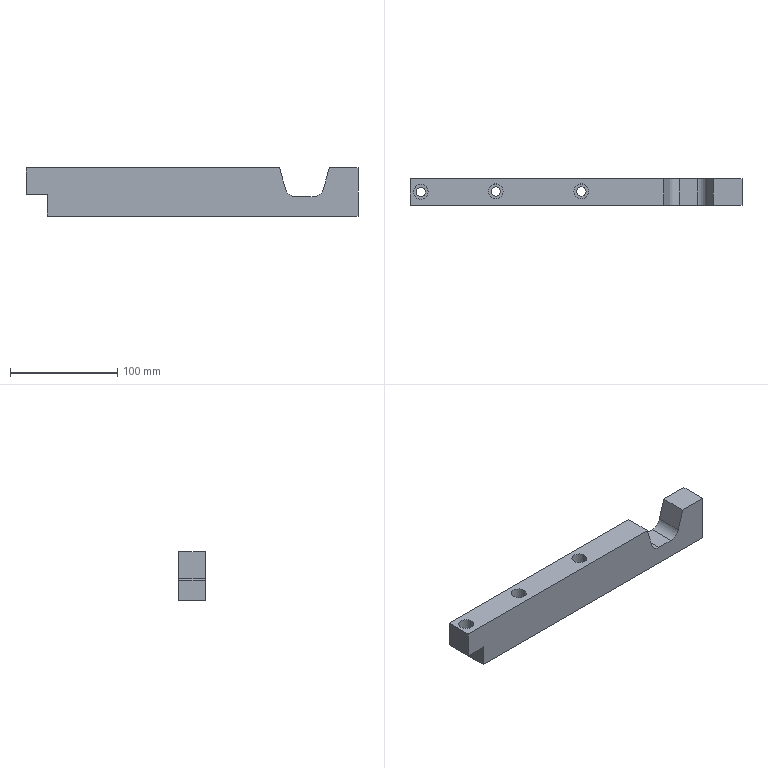Part | STEP file | 冲床-300配套压波_id986_x_t | 1 solid | 26 faces | box 310 x 25 x 45 mm | volume 301509 mm3 | plane 15 | cylinder 11 | commonest cylinder face diameters 8.7 x3 14 x3 4 x2 20 x2 1 x1
STEP:
#1=CARTESIAN_POINT('',(1952.,-82.5,-185.));
#2=VERTEX_POINT('',#1);
#3=CARTESIAN_POINT('',(1945.,-82.5,-185.));
#4=DIRECTION('',(0.,0.,-1.));
#5=DIRECTION('',(1.,0.,0.));
#6=AXIS2_PLACEMENT_3D('',#3,#4,#5);
#7=CIRCLE('',#6,7.);
#8=EDGE_CURVE('',#2,#2,#7,.T.);
#9=ORIENTED_EDGE('',*,*,#8,.T.);
#10=EDGE_LOOP('',(#9));
#11=FACE_BOUND('',#10,.T.);
#12=CARTESIAN_POINT('',(2102.,-82.01,-185.));
#13=VERTEX_POINT('',#12);
#14=CARTESIAN_POINT('',(2095.,-82.01,-185.));
#15=DIRECTION('',(0.,0.,-1.));
#16=DIRECTION('',(1.,0.,0.));
#17=AXIS2_PLACEMENT_3D('',#14,#15,#16);
#18=CIRCLE('',#17,7.);
#19=EDGE_CURVE('',#13,#13,#18,.T.);
#20=ORIENTED_EDGE('',*,*,#19,.T.);
#21=EDGE_LOOP('',(#20));
#22=FACE_BOUND('',#21,.T.);
#23=CARTESIAN_POINT('',(2022.,-82.01,-185.));
#24=VERTEX_POINT('',#23);
#25=CARTESIAN_POINT('',(2015.,-82.01,-185.));
#26=DIRECTION('',(0.,0.,-1.));
#27=DIRECTION('',(1.,0.,0.));
#28=AXIS2_PLACEMENT_3D('',#25,#26,#27);
#29=CIRCLE('',#28,7.);
#30=EDGE_CURVE('',#24,#24,#29,.T.);
#31=ORIENTED_EDGE('',*,*,#30,.T.);
#32=EDGE_LOOP('',(#31));
#33=FACE_BOUND('',#32,.T.);
#34=CARTESIAN_POINT('',(2171.709,-95.,-185.));
#35=VERTEX_POINT('',#34);
#36=CARTESIAN_POINT('',(1935.,-95.,-185.));
#37=VERTEX_POINT('',#36);
#38=CARTESIAN_POINT('',(1985.,-95.,-185.));
#39=DIRECTION('',(-1.,0.,0.));
#40=VECTOR('',#39,1.);
#41=LINE('',#38,#40);
#42=EDGE_CURVE('',#35,#37,#41,.T.);
#43=ORIENTED_EDGE('',*,*,#42,.F.);
#44=CARTESIAN_POINT('',(2171.709,-70.,-185.));
#45=VERTEX_POINT('',#44);
#46=CARTESIAN_POINT('',(2171.709,-298.,-185.));
#47=DIRECTION('',(0.,1.,0.));
#48=VECTOR('',#47,1.);
#49=LINE('',#46,#48);
#50=EDGE_CURVE('',#35,#45,#49,.T.);
#51=ORIENTED_EDGE('',*,*,#50,.T.);
#52=CARTESIAN_POINT('',(1935.,-70.,-185.));
#53=VERTEX_POINT('',#52);
#54=CARTESIAN_POINT('',(2135.,-70.,-185.));
#55=DIRECTION('',(-1.,0.,0.));
#56=VECTOR('',#55,1.);
#57=LINE('',#54,#56);
#58=EDGE_CURVE('',#45,#53,#57,.T.);
#59=ORIENTED_EDGE('',*,*,#58,.T.);
#60=CARTESIAN_POINT('',(1935.,-298.,-185.));
#61=DIRECTION('',(0.,-1.,0.));
#62=VECTOR('',#61,1.);
#63=LINE('',#60,#62);
#64=EDGE_CURVE('',#53,#37,#63,.T.);
#65=ORIENTED_EDGE('',*,*,#64,.T.);
#66=EDGE_LOOP('',(#43,#51,#59,#65));
#67=FACE_BOUND('',#66,.T.);
#68=CARTESIAN_POINT('',(1985.,-298.,-185.));
#69=DIRECTION('',(0.,0.,1.));
#70=DIRECTION('',(1.,0.,0.));
#71=AXIS2_PLACEMENT_3D('',#68,#69,#70);
#72=PLANE('',#71);
#73=ADVANCED_FACE('',(#11,#22,#33,#67),#72,.T.);
#74=CARTESIAN_POINT('',(2245.,-95.,-185.));
#75=VERTEX_POINT('',#74);
#76=CARTESIAN_POINT('',(2245.,-70.,-185.));
#77=VERTEX_POINT('',#76);
#78=CARTESIAN_POINT('',(2245.,-298.,-185.));
#79=DIRECTION('',(0.,1.,0.));
#80=VECTOR('',#79,1.);
#81=LINE('',#78,#80);
#82=EDGE_CURVE('',#75,#77,#81,.T.);
#83=ORIENTED_EDGE('',*,*,#82,.T.);
#84=CARTESIAN_POINT('',(2218.291,-70.,-185.));
#85=VERTEX_POINT('',#84);
#86=CARTESIAN_POINT('',(2135.,-70.,-185.));
#87=DIRECTION('',(-1.,0.,0.));
#88=VECTOR('',#87,1.);
#89=LINE('',#86,#88);
#90=EDGE_CURVE('',#77,#85,#89,.T.);
#91=ORIENTED_EDGE('',*,*,#90,.T.);
#92=CARTESIAN_POINT('',(2218.291,-95.,-185.));
#93=VERTEX_POINT('',#92);
#94=CARTESIAN_POINT('',(2218.291,-298.,-185.));
#95=DIRECTION('',(0.,-1.,0.));
#96=VECTOR('',#95,1.);
#97=LINE('',#94,#96);
#98=EDGE_CURVE('',#85,#93,#97,.T.);
#99=ORIENTED_EDGE('',*,*,#98,.T.);
#100=CARTESIAN_POINT('',(1975.,-95.,-185.));
#101=DIRECTION('',(-1.,0.,0.));
#102=VECTOR('',#101,1.);
#103=LINE('',#100,#102);
#104=EDGE_CURVE('',#75,#93,#103,.T.);
#105=ORIENTED_EDGE('',*,*,#104,.F.);
#106=EDGE_LOOP('',(#83,#91,#99,#105));
#107=FACE_OUTER_BOUND('',#106,.T.);
#108=CARTESIAN_POINT('',(1975.,-298.,-185.));
#109=DIRECTION('',(0.,0.,1.));
#110=DIRECTION('',(1.,0.,0.));
#111=AXIS2_PLACEMENT_3D('',#108,#109,#110);
#112=PLANE('',#111);
#113=ADVANCED_FACE('',(#107),#112,.T.);
#114=CARTESIAN_POINT('',(2245.,-95.,-230.));
#115=VERTEX_POINT('',#114);
#116=CARTESIAN_POINT('',(2245.,-70.,-230.));
#117=VERTEX_POINT('',#116);
#118=CARTESIAN_POINT('',(2245.,-298.,-230.));
#119=DIRECTION('',(0.,1.,0.));
#120=VECTOR('',#119,1.);
#121=LINE('',#118,#120);
#122=EDGE_CURVE('',#115,#117,#121,.T.);
#123=ORIENTED_EDGE('',*,*,#122,.T.);
#124=CARTESIAN_POINT('',(2245.,-70.,-390.));
#125=DIRECTION('',(0.,0.,1.));
#126=VECTOR('',#125,1.);
#127=LINE('',#124,#126);
#128=EDGE_CURVE('',#117,#77,#127,.T.);
#129=ORIENTED_EDGE('',*,*,#128,.T.);
#130=ORIENTED_EDGE('',*,*,#82,.F.);
#131=CARTESIAN_POINT('',(2245.,-95.,-190.));
#132=DIRECTION('',(0.,0.,1.));
#133=VECTOR('',#132,1.);
#134=LINE('',#131,#133);
#135=EDGE_CURVE('',#115,#75,#134,.T.);
#136=ORIENTED_EDGE('',*,*,#135,.F.);
#137=EDGE_LOOP('',(#123,#129,#130,#136));
#138=FACE_OUTER_BOUND('',#137,.T.);
#139=CARTESIAN_POINT('',(2245.,-298.,-190.));
#140=DIRECTION('',(1.,0.,0.));
#141=DIRECTION('',(0.,1.,0.));
#142=AXIS2_PLACEMENT_3D('',#139,#140,#141);
#143=PLANE('',#142);
#144=ADVANCED_FACE('',(#138),#143,.T.);
#145=CARTESIAN_POINT('',(1955.,-70.,-230.));
#146=VERTEX_POINT('',#145);
#147=CARTESIAN_POINT('',(1985.,-70.,-230.));
#148=DIRECTION('',(1.,0.,0.));
#149=VECTOR('',#148,1.);
#150=LINE('',#147,#149);
#151=EDGE_CURVE('',#146,#117,#150,.T.);
#152=ORIENTED_EDGE('',*,*,#151,.T.);
#153=ORIENTED_EDGE('',*,*,#122,.F.);
#154=CARTESIAN_POINT('',(1955.,-95.,-230.));
#155=VERTEX_POINT('',#154);
#156=CARTESIAN_POINT('',(1985.,-95.,-230.));
#157=DIRECTION('',(-1.,0.,0.));
#158=VECTOR('',#157,1.);
#159=LINE('',#156,#158);
#160=EDGE_CURVE('',#115,#155,#159,.T.);
#161=ORIENTED_EDGE('',*,*,#160,.T.);
#162=CARTESIAN_POINT('',(1955.,-80.,-230.));
#163=DIRECTION('',(0.,-1.,0.));
#164=VECTOR('',#163,1.);
#165=LINE('',#162,#164);
#166=EDGE_CURVE('',#146,#155,#165,.T.);
#167=ORIENTED_EDGE('',*,*,#166,.F.);
#168=EDGE_LOOP('',(#152,#153,#161,#167));
#169=FACE_BOUND('',#168,.T.);
#170=CARTESIAN_POINT('',(2019.35,-82.01,-230.));
#171=VERTEX_POINT('',#170);
#172=CARTESIAN_POINT('',(2015.,-82.01,-230.));
#173=DIRECTION('',(0.,0.,1.));
#174=DIRECTION('',(1.,0.,0.));
#175=AXIS2_PLACEMENT_3D('',#172,#173,#174);
#176=CIRCLE('',#175,4.35);
#177=EDGE_CURVE('',#171,#171,#176,.T.);
#178=ORIENTED_EDGE('',*,*,#177,.T.);
#179=EDGE_LOOP('',(#178));
#180=FACE_BOUND('',#179,.T.);
#181=CARTESIAN_POINT('',(2099.35,-82.01,-230.));
#182=VERTEX_POINT('',#181);
#183=CARTESIAN_POINT('',(2095.,-82.01,-230.));
#184=DIRECTION('',(0.,0.,1.));
#185=DIRECTION('',(1.,0.,0.));
#186=AXIS2_PLACEMENT_3D('',#183,#184,#185);
#187=CIRCLE('',#186,4.35);
#188=EDGE_CURVE('',#182,#182,#187,.T.);
#189=ORIENTED_EDGE('',*,*,#188,.T.);
#190=EDGE_LOOP('',(#189));
#191=FACE_BOUND('',#190,.T.);
#192=CARTESIAN_POINT('',(1985.,-298.,-230.));
#193=DIRECTION('',(0.,0.,1.));
#194=DIRECTION('',(1.,0.,0.));
#195=AXIS2_PLACEMENT_3D('',#192,#193,#194);
#196=PLANE('',#195);
#197=ADVANCED_FACE('',(#169,#180,#191),#196,.F.);
#198=CARTESIAN_POINT('',(1955.,-95.,-211.5));
#199=VERTEX_POINT('',#198);
#200=CARTESIAN_POINT('',(1955.,-95.,-70.));
#201=DIRECTION('',(0.,0.,1.));
#202=VECTOR('',#201,1.);
#203=LINE('',#200,#202);
#204=EDGE_CURVE('',#155,#199,#203,.T.);
#205=ORIENTED_EDGE('',*,*,#204,.T.);
#206=CARTESIAN_POINT('',(1955.,-70.,-211.5));
#207=VERTEX_POINT('',#206);
#208=CARTESIAN_POINT('',(1955.,0.,-211.5));
#209=DIRECTION('',(0.,1.,0.));
#210=VECTOR('',#209,1.);
#211=LINE('',#208,#210);
#212=EDGE_CURVE('',#199,#207,#211,.T.);
#213=ORIENTED_EDGE('',*,*,#212,.T.);
#214=CARTESIAN_POINT('',(1955.,-70.,-390.));
#215=DIRECTION('',(0.,0.,-1.));
#216=VECTOR('',#215,1.);
#217=LINE('',#214,#216);
#218=EDGE_CURVE('',#207,#146,#217,.T.);
#219=ORIENTED_EDGE('',*,*,#218,.T.);
#220=ORIENTED_EDGE('',*,*,#166,.T.);
#221=EDGE_LOOP('',(#205,#213,#219,#220));
#222=FACE_OUTER_BOUND('',#221,.T.);
#223=CARTESIAN_POINT('',(1955.,0.,-312.5));
#224=DIRECTION('',(-1.,0.,0.));
#225=DIRECTION('',(0.,0.,1.));
#226=AXIS2_PLACEMENT_3D('',#223,#224,#225);
#227=PLANE('',#226);
#228=ADVANCED_FACE('',(#222),#227,.T.);
#229=CARTESIAN_POINT('',(2212.604,-70.,-204.765));
#230=VERTEX_POINT('',#229);
#231=CARTESIAN_POINT('',(2225.867,-70.,-158.668));
#232=DIRECTION('',(-0.2765,0.,-0.961));
#233=VECTOR('',#232,1.);
#234=LINE('',#231,#233);
#235=EDGE_CURVE('',#85,#230,#234,.T.);
#236=ORIENTED_EDGE('',*,*,#235,.F.);
#237=ORIENTED_EDGE('',*,*,#90,.F.);
#238=ORIENTED_EDGE('',*,*,#128,.F.);
#239=ORIENTED_EDGE('',*,*,#151,.F.);
#240=ORIENTED_EDGE('',*,*,#218,.F.);
#241=CARTESIAN_POINT('',(1955.4,-70.,-210.3));
#242=VERTEX_POINT('',#241);
#243=CARTESIAN_POINT('',(1957.,-70.,-211.5));
#244=DIRECTION('',(0.,1.,0.));
#245=DIRECTION('',(0.,0.,-1.));
#246=AXIS2_PLACEMENT_3D('',#243,#244,#245);
#247=CIRCLE('',#246,2.);
#248=EDGE_CURVE('',#207,#242,#247,.T.);
#249=ORIENTED_EDGE('',*,*,#248,.T.);
#250=CARTESIAN_POINT('',(1954.7,-70.,-209.6));
#251=VERTEX_POINT('',#250);
#252=CARTESIAN_POINT('',(1955.,-70.,-210.));
#253=DIRECTION('',(0.,1.,0.));
#254=DIRECTION('',(-1.,0.,0.));
#255=AXIS2_PLACEMENT_3D('',#252,#253,#254);
#256=CIRCLE('',#255,0.5);
#257=EDGE_CURVE('',#251,#242,#256,.T.);
#258=ORIENTED_EDGE('',*,*,#257,.F.);
#259=CARTESIAN_POINT('',(1953.5,-70.,-210.));
#260=VERTEX_POINT('',#259);
#261=CARTESIAN_POINT('',(1953.5,-70.,-208.));
#262=DIRECTION('',(0.,1.,0.));
#263=DIRECTION('',(0.,0.,-1.));
#264=AXIS2_PLACEMENT_3D('',#261,#262,#263);
#265=CIRCLE('',#264,2.);
#266=EDGE_CURVE('',#251,#260,#265,.T.);
#267=ORIENTED_EDGE('',*,*,#266,.T.);
#268=CARTESIAN_POINT('',(1935.,-70.,-210.));
#269=VERTEX_POINT('',#268);
#270=CARTESIAN_POINT('',(1955.,-70.,-210.));
#271=DIRECTION('',(-1.,0.,0.));
#272=VECTOR('',#271,1.);
#273=LINE('',#270,#272);
#274=EDGE_CURVE('',#260,#269,#273,.T.);
#275=ORIENTED_EDGE('',*,*,#274,.T.);
#276=CARTESIAN_POINT('',(1935.,-70.,-185.));
#277=DIRECTION('',(0.,0.,-1.));
#278=VECTOR('',#277,1.);
#279=LINE('',#276,#278);
#280=EDGE_CURVE('',#53,#269,#279,.T.);
#281=ORIENTED_EDGE('',*,*,#280,.F.);
#282=ORIENTED_EDGE('',*,*,#58,.F.);
#283=CARTESIAN_POINT('',(2177.396,-70.,-204.765));
#284=VERTEX_POINT('',#283);
#285=CARTESIAN_POINT('',(2180.341,-70.,-215.));
#286=DIRECTION('',(-0.2765,0.,0.961));
#287=VECTOR('',#286,1.);
#288=LINE('',#285,#287);
#289=EDGE_CURVE('',#284,#45,#288,.T.);
#290=ORIENTED_EDGE('',*,*,#289,.F.);
#291=CARTESIAN_POINT('',(2187.006,-70.,-212.));
#292=VERTEX_POINT('',#291);
#293=CARTESIAN_POINT('',(2187.006,-70.,-202.));
#294=DIRECTION('',(0.,-1.,0.));
#295=DIRECTION('',(0.,0.,-1.));
#296=AXIS2_PLACEMENT_3D('',#293,#294,#295);
#297=CIRCLE('',#296,10.);
#298=EDGE_CURVE('',#284,#292,#297,.T.);
#299=ORIENTED_EDGE('',*,*,#298,.T.);
#300=CARTESIAN_POINT('',(2202.994,-70.,-212.));
#301=VERTEX_POINT('',#300);
#302=CARTESIAN_POINT('',(2135.,-70.,-212.));
#303=DIRECTION('',(-1.,0.,0.));
#304=VECTOR('',#303,1.);
#305=LINE('',#302,#304);
#306=EDGE_CURVE('',#301,#292,#305,.T.);
#307=ORIENTED_EDGE('',*,*,#306,.F.);
#308=CARTESIAN_POINT('',(2202.994,-70.,-202.));
#309=DIRECTION('',(0.,-1.,0.));
#310=DIRECTION('',(0.,0.,-1.));
#311=AXIS2_PLACEMENT_3D('',#308,#309,#310);
#312=CIRCLE('',#311,10.);
#313=EDGE_CURVE('',#301,#230,#312,.T.);
#314=ORIENTED_EDGE('',*,*,#313,.T.);
#315=EDGE_LOOP('',(#236,#237,#238,#239,#240,#249,#258,#267,#275,#281,#282,#290,#299,#307,#314));
#316=FACE_OUTER_BOUND('',#315,.T.);
#317=CARTESIAN_POINT('',(2135.,-70.,-390.));
#318=DIRECTION('',(0.,-1.,0.));
#319=DIRECTION('',(0.,0.,-1.));
#320=AXIS2_PLACEMENT_3D('',#317,#318,#319);
#321=PLANE('',#320);
#322=ADVANCED_FACE('',(#316),#321,.F.);
#323=ORIENTED_EDGE('',*,*,#104,.T.);
#324=CARTESIAN_POINT('',(2212.604,-95.,-204.765));
#325=VERTEX_POINT('',#324);
#326=CARTESIAN_POINT('',(2312.487,-95.,142.39));
#327=DIRECTION('',(-0.2765,0.,-0.961));
#328=VECTOR('',#327,1.);
#329=LINE('',#326,#328);
#330=EDGE_CURVE('',#93,#325,#329,.T.);
#331=ORIENTED_EDGE('',*,*,#330,.T.);
#332=CARTESIAN_POINT('',(2202.994,-95.,-212.));
#333=VERTEX_POINT('',#332);
#334=CARTESIAN_POINT('',(2202.994,-95.,-202.));
#335=DIRECTION('',(0.,1.,0.));
#336=DIRECTION('',(0.,0.,1.));
#337=AXIS2_PLACEMENT_3D('',#334,#335,#336);
#338=CIRCLE('',#337,10.);
#339=EDGE_CURVE('',#325,#333,#338,.T.);
#340=ORIENTED_EDGE('',*,*,#339,.T.);
#341=CARTESIAN_POINT('',(2187.006,-95.,-212.));
#342=VERTEX_POINT('',#341);
#343=CARTESIAN_POINT('',(2195.,-95.,-212.));
#344=DIRECTION('',(-1.,0.,0.));
#345=VECTOR('',#344,1.);
#346=LINE('',#343,#345);
#347=EDGE_CURVE('',#333,#342,#346,.T.);
#348=ORIENTED_EDGE('',*,*,#347,.T.);
#349=CARTESIAN_POINT('',(2177.396,-95.,-204.765));
#350=VERTEX_POINT('',#349);
#351=CARTESIAN_POINT('',(2187.006,-95.,-202.));
#352=DIRECTION('',(0.,1.,0.));
#353=DIRECTION('',(0.,0.,1.));
#354=AXIS2_PLACEMENT_3D('',#351,#352,#353);
#355=CIRCLE('',#354,10.);
#356=EDGE_CURVE('',#342,#350,#355,.T.);
#357=ORIENTED_EDGE('',*,*,#356,.T.);
#358=CARTESIAN_POINT('',(2164.133,-95.,-158.668));
#359=DIRECTION('',(-0.2765,0.,0.961));
#360=VECTOR('',#359,1.);
#361=LINE('',#358,#360);
#362=EDGE_CURVE('',#350,#35,#361,.T.);
#363=ORIENTED_EDGE('',*,*,#362,.T.);
#364=ORIENTED_EDGE('',*,*,#42,.T.);
#365=CARTESIAN_POINT('',(1935.,-95.,-210.));
#366=VERTEX_POINT('',#365);
#367=CARTESIAN_POINT('',(1935.,-95.,-185.));
#368=DIRECTION('',(0.,0.,-1.));
#369=VECTOR('',#368,1.);
#370=LINE('',#367,#369);
#371=EDGE_CURVE('',#37,#366,#370,.T.);
#372=ORIENTED_EDGE('',*,*,#371,.T.);
#373=CARTESIAN_POINT('',(1953.5,-95.,-210.));
#374=VERTEX_POINT('',#373);
#375=CARTESIAN_POINT('',(1975.,-95.,-210.));
#376=DIRECTION('',(-1.,0.,0.));
#377=VECTOR('',#376,1.);
#378=LINE('',#375,#377);
#379=EDGE_CURVE('',#374,#366,#378,.T.);
#380=ORIENTED_EDGE('',*,*,#379,.F.);
#381=CARTESIAN_POINT('',(1954.7,-95.,-209.6));
#382=VERTEX_POINT('',#381);
#383=CARTESIAN_POINT('',(1953.5,-95.,-208.));
#384=DIRECTION('',(0.,-1.,0.));
#385=DIRECTION('',(0.,0.,1.));
#386=AXIS2_PLACEMENT_3D('',#383,#384,#385);
#387=CIRCLE('',#386,2.);
#388=EDGE_CURVE('',#374,#382,#387,.T.);
#389=ORIENTED_EDGE('',*,*,#388,.T.);
#390=CARTESIAN_POINT('',(1955.4,-95.,-210.3));
#391=VERTEX_POINT('',#390);
#392=CARTESIAN_POINT('',(1955.,-95.,-210.));
#393=DIRECTION('',(0.,-1.,0.));
#394=DIRECTION('',(-1.,0.,0.));
#395=AXIS2_PLACEMENT_3D('',#392,#393,#394);
#396=CIRCLE('',#395,0.5);
#397=EDGE_CURVE('',#391,#382,#396,.T.);
#398=ORIENTED_EDGE('',*,*,#397,.F.);
#399=CARTESIAN_POINT('',(1957.,-95.,-211.5));
#400=DIRECTION('',(0.,-1.,0.));
#401=DIRECTION('',(0.,0.,1.));
#402=AXIS2_PLACEMENT_3D('',#399,#400,#401);
#403=CIRCLE('',#402,2.);
#404=EDGE_CURVE('',#391,#199,#403,.T.);
#405=ORIENTED_EDGE('',*,*,#404,.T.);
#406=ORIENTED_EDGE('',*,*,#204,.F.);
#407=ORIENTED_EDGE('',*,*,#160,.F.);
#408=ORIENTED_EDGE('',*,*,#135,.T.);
#409=EDGE_LOOP('',(#323,#331,#340,#348,#357,#363,#364,#372,#380,#389,#398,#405,#406,#407,#408));
#410=FACE_OUTER_BOUND('',#409,.T.);
#411=CARTESIAN_POINT('',(1975.,-95.,-70.));
#412=DIRECTION('',(0.,1.,0.));
#413=DIRECTION('',(0.,0.,1.));
#414=AXIS2_PLACEMENT_3D('',#411,#412,#413);
#415=PLANE('',#414);
#416=ADVANCED_FACE('',(#410),#415,.F.);
#417=CARTESIAN_POINT('',(1940.65,-82.5,-210.));
#418=VERTEX_POINT('',#417);
#419=CARTESIAN_POINT('',(1945.,-82.5,-210.));
#420=DIRECTION('',(0.,0.,-1.));
#421=DIRECTION('',(-1.,0.,0.));
#422=AXIS2_PLACEMENT_3D('',#419,#420,#421);
#423=CIRCLE('',#422,4.35);
#424=EDGE_CURVE('',#418,#418,#423,.T.);
#425=ORIENTED_EDGE('',*,*,#424,.F.);
#426=EDGE_LOOP('',(#425));
#427=FACE_BOUND('',#426,.T.);
#428=ORIENTED_EDGE('',*,*,#274,.F.);
#429=CARTESIAN_POINT('',(1953.5,-70.,-210.));
#430=DIRECTION('',(0.,-1.,0.));
#431=VECTOR('',#430,1.);
#432=LINE('',#429,#431);
#433=EDGE_CURVE('',#260,#374,#432,.T.);
#434=ORIENTED_EDGE('',*,*,#433,.T.);
#435=ORIENTED_EDGE('',*,*,#379,.T.);
#436=CARTESIAN_POINT('',(1935.,-70.,-210.));
#437=DIRECTION('',(0.,-1.,0.));
#438=VECTOR('',#437,1.);
#439=LINE('',#436,#438);
#440=EDGE_CURVE('',#269,#366,#439,.T.);
#441=ORIENTED_EDGE('',*,*,#440,.F.);
#442=EDGE_LOOP('',(#428,#434,#435,#441));
#443=FACE_BOUND('',#442,.T.);
#444=CARTESIAN_POINT('',(1955.,-70.,-210.));
#445=DIRECTION('',(0.,0.,-1.));
#446=DIRECTION('',(-1.,0.,0.));
#447=AXIS2_PLACEMENT_3D('',#444,#445,#446);
#448=PLANE('',#447);
#449=ADVANCED_FACE('',(#427,#443),#448,.T.);
#450=CARTESIAN_POINT('',(2090.65,-82.01,-205.));
#451=VERTEX_POINT('',#450);
#452=CARTESIAN_POINT('',(2095.,-82.01,-205.));
#453=DIRECTION('',(0.,0.,1.));
#454=DIRECTION('',(-1.,0.,0.));
#455=AXIS2_PLACEMENT_3D('',#452,#453,#454);
#456=CIRCLE('',#455,4.35);
#457=EDGE_CURVE('',#451,#451,#456,.T.);
#458=ORIENTED_EDGE('',*,*,#457,.F.);
#459=EDGE_LOOP('',(#458));
#460=FACE_BOUND('',#459,.T.);
#461=CARTESIAN_POINT('',(2088.,-82.01,-205.));
#462=VERTEX_POINT('',#461);
#463=CARTESIAN_POINT('',(2095.,-82.01,-205.));
#464=DIRECTION('',(0.,0.,1.));
#465=DIRECTION('',(-1.,0.,0.));
#466=AXIS2_PLACEMENT_3D('',#463,#464,#465);
#467=CIRCLE('',#466,7.);
#468=EDGE_CURVE('',#462,#462,#467,.T.);
#469=ORIENTED_EDGE('',*,*,#468,.T.);
#470=EDGE_LOOP('',(#469));
#471=FACE_BOUND('',#470,.T.);
#472=CARTESIAN_POINT('',(2095.,-82.01,-205.));
#473=DIRECTION('',(0.,0.,-1.));
#474=DIRECTION('',(-1.,0.,0.));
#475=AXIS2_PLACEMENT_3D('',#472,#473,#474);
#476=PLANE('',#475);
#477=ADVANCED_FACE('',(#460,#471),#476,.F.);
#478=ORIENTED_EDGE('',*,*,#19,.F.);
#479=EDGE_LOOP('',(#478));
#480=FACE_BOUND('',#479,.T.);
#481=ORIENTED_EDGE('',*,*,#468,.F.);
#482=EDGE_LOOP('',(#481));
#483=FACE_BOUND('',#482,.T.);
#484=CARTESIAN_POINT('',(2095.,-82.01,-185.));
#485=DIRECTION('',(0.,0.,-1.));
#486=DIRECTION('',(-1.,0.,0.));
#487=AXIS2_PLACEMENT_3D('',#484,#485,#486);
#488=CYLINDRICAL_SURFACE('',#487,7.);
#489=ADVANCED_FACE('',(#480,#483),#488,.F.);
#490=ORIENTED_EDGE('',*,*,#330,.F.);
#491=ORIENTED_EDGE('',*,*,#98,.F.);
#492=ORIENTED_EDGE('',*,*,#235,.T.);
#493=CARTESIAN_POINT('',(2212.604,-95.,-204.765));
#494=DIRECTION('',(0.,-1.,0.));
#495=VECTOR('',#494,1.);
#496=LINE('',#493,#495);
#497=EDGE_CURVE('',#230,#325,#496,.T.);
#498=ORIENTED_EDGE('',*,*,#497,.T.);
#499=EDGE_LOOP('',(#490,#491,#492,#498));
#500=FACE_OUTER_BOUND('',#499,.T.);
#501=CARTESIAN_POINT('',(2312.487,-70.,142.39));
#502=DIRECTION('',(-0.961,0.,0.2765));
#503=DIRECTION('',(0.2765,0.,0.961));
#504=AXIS2_PLACEMENT_3D('',#501,#502,#503);
#505=PLANE('',#504);
#506=ADVANCED_FACE('',(#500),#505,.T.);
#507=ORIENTED_EDGE('',*,*,#289,.T.);
#508=ORIENTED_EDGE('',*,*,#50,.F.);
#509=ORIENTED_EDGE('',*,*,#362,.F.);
#510=CARTESIAN_POINT('',(2177.396,-70.,-204.765));
#511=DIRECTION('',(0.,1.,0.));
#512=VECTOR('',#511,1.);
#513=LINE('',#510,#512);
#514=EDGE_CURVE('',#350,#284,#513,.T.);
#515=ORIENTED_EDGE('',*,*,#514,.T.);
#516=EDGE_LOOP('',(#507,#508,#509,#515));
#517=FACE_OUTER_BOUND('',#516,.T.);
#518=CARTESIAN_POINT('',(2164.133,-70.,-158.668));
#519=DIRECTION('',(0.961,0.,0.2765));
#520=DIRECTION('',(0.2765,0.,-0.961));
#521=AXIS2_PLACEMENT_3D('',#518,#519,#520);
#522=PLANE('',#521);
#523=ADVANCED_FACE('',(#517),#522,.T.);
#524=ORIENTED_EDGE('',*,*,#347,.F.);
#525=CARTESIAN_POINT('',(2202.994,-70.,-212.));
#526=DIRECTION('',(0.,1.,0.));
#527=VECTOR('',#526,1.);
#528=LINE('',#525,#527);
#529=EDGE_CURVE('',#333,#301,#528,.T.);
#530=ORIENTED_EDGE('',*,*,#529,.T.);
#531=ORIENTED_EDGE('',*,*,#306,.T.);
#532=CARTESIAN_POINT('',(2187.006,-95.,-212.));
#533=DIRECTION('',(0.,-1.,0.));
#534=VECTOR('',#533,1.);
#535=LINE('',#532,#534);
#536=EDGE_CURVE('',#292,#342,#535,.T.);
#537=ORIENTED_EDGE('',*,*,#536,.T.);
#538=EDGE_LOOP('',(#524,#530,#531,#537));
#539=FACE_OUTER_BOUND('',#538,.T.);
#540=CARTESIAN_POINT('',(2195.,-70.,-212.));
#541=DIRECTION('',(0.,0.,1.));
#542=DIRECTION('',(1.,0.,0.));
#543=AXIS2_PLACEMENT_3D('',#540,#541,#542);
#544=PLANE('',#543);
#545=ADVANCED_FACE('',(#539),#544,.T.);
#546=ORIENTED_EDGE('',*,*,#371,.F.);
#547=ORIENTED_EDGE('',*,*,#64,.F.);
#548=ORIENTED_EDGE('',*,*,#280,.T.);
#549=ORIENTED_EDGE('',*,*,#440,.T.);
#550=EDGE_LOOP('',(#546,#547,#548,#549));
#551=FACE_OUTER_BOUND('',#550,.T.);
#552=CARTESIAN_POINT('',(1935.,-70.,-185.));
#553=DIRECTION('',(1.,0.,0.));
#554=DIRECTION('',(0.,-1.,0.));
#555=AXIS2_PLACEMENT_3D('',#552,#553,#554);
#556=PLANE('',#555);
#557=ADVANCED_FACE('',(#551),#556,.F.);
#558=CARTESIAN_POINT('',(2010.65,-82.01,-205.));
#559=VERTEX_POINT('',#558);
#560=CARTESIAN_POINT('',(2015.,-82.01,-205.));
#561=DIRECTION('',(0.,0.,1.));
#562=DIRECTION('',(-1.,0.,0.));
#563=AXIS2_PLACEMENT_3D('',#560,#561,#562);
#564=CIRCLE('',#563,4.35);
#565=EDGE_CURVE('',#559,#559,#564,.T.);
#566=ORIENTED_EDGE('',*,*,#565,.T.);
#567=EDGE_LOOP('',(#566));
#568=FACE_BOUND('',#567,.T.);
#569=ORIENTED_EDGE('',*,*,#177,.F.);
#570=EDGE_LOOP('',(#569));
#571=FACE_BOUND('',#570,.T.);
#572=CARTESIAN_POINT('',(2015.,-82.01,-235.));
#573=DIRECTION('',(0.,0.,-1.));
#574=DIRECTION('',(-1.,0.,0.));
#575=AXIS2_PLACEMENT_3D('',#572,#573,#574);
#576=CYLINDRICAL_SURFACE('',#575,4.35);
#577=ADVANCED_FACE('',(#568,#571),#576,.F.);
#578=ORIENTED_EDGE('',*,*,#565,.F.);
#579=EDGE_LOOP('',(#578));
#580=FACE_BOUND('',#579,.T.);
#581=CARTESIAN_POINT('',(2008.,-82.01,-205.));
#582=VERTEX_POINT('',#581);
#583=CARTESIAN_POINT('',(2015.,-82.01,-205.));
#584=DIRECTION('',(0.,0.,1.));
#585=DIRECTION('',(-1.,0.,0.));
#586=AXIS2_PLACEMENT_3D('',#583,#584,#585);
#587=CIRCLE('',#586,7.);
#588=EDGE_CURVE('',#582,#582,#587,.T.);
#589=ORIENTED_EDGE('',*,*,#588,.T.);
#590=EDGE_LOOP('',(#589));
#591=FACE_BOUND('',#590,.T.);
#592=CARTESIAN_POINT('',(2015.,-82.01,-205.));
#593=DIRECTION('',(0.,0.,-1.));
#594=DIRECTION('',(-1.,0.,0.));
#595=AXIS2_PLACEMENT_3D('',#592,#593,#594);
#596=PLANE('',#595);
#597=ADVANCED_FACE('',(#580,#591),#596,.F.);
#598=ORIENTED_EDGE('',*,*,#588,.F.);
#599=EDGE_LOOP('',(#598));
#600=FACE_BOUND('',#599,.T.);
#601=ORIENTED_EDGE('',*,*,#30,.F.);
#602=EDGE_LOOP('',(#601));
#603=FACE_BOUND('',#602,.T.);
#604=CARTESIAN_POINT('',(2015.,-82.01,-185.));
#605=DIRECTION('',(0.,0.,-1.));
#606=DIRECTION('',(-1.,0.,0.));
#607=AXIS2_PLACEMENT_3D('',#604,#605,#606);
#608=CYLINDRICAL_SURFACE('',#607,7.);
#609=ADVANCED_FACE('',(#600,#603),#608,.F.);
#610=ORIENTED_EDGE('',*,*,#457,.T.);
#611=EDGE_LOOP('',(#610));
#612=FACE_BOUND('',#611,.T.);
#613=ORIENTED_EDGE('',*,*,#188,.F.);
#614=EDGE_LOOP('',(#613));
#615=FACE_BOUND('',#614,.T.);
#616=CARTESIAN_POINT('',(2095.,-82.01,-235.));
#617=DIRECTION('',(0.,0.,-1.));
#618=DIRECTION('',(-1.,0.,0.));
#619=AXIS2_PLACEMENT_3D('',#616,#617,#618);
#620=CYLINDRICAL_SURFACE('',#619,4.35);
#621=ADVANCED_FACE('',(#612,#615),#620,.F.);
#622=ORIENTED_EDGE('',*,*,#424,.T.);
#623=EDGE_LOOP('',(#622));
#624=FACE_BOUND('',#623,.T.);
#625=CARTESIAN_POINT('',(1940.65,-82.5,-195.));
#626=VERTEX_POINT('',#625);
#627=CARTESIAN_POINT('',(1945.,-82.5,-195.));
#628=DIRECTION('',(0.,0.,1.));
#629=DIRECTION('',(-1.,0.,0.));
#630=AXIS2_PLACEMENT_3D('',#627,#628,#629);
#631=CIRCLE('',#630,4.35);
#632=EDGE_CURVE('',#626,#626,#631,.T.);
#633=ORIENTED_EDGE('',*,*,#632,.T.);
#634=EDGE_LOOP('',(#633));
#635=FACE_BOUND('',#634,.T.);
#636=CARTESIAN_POINT('',(1945.,-82.5,-301.999));
#637=DIRECTION('',(0.,0.,-1.));
#638=DIRECTION('',(-1.,0.,0.));
#639=AXIS2_PLACEMENT_3D('',#636,#637,#638);
#640=CYLINDRICAL_SURFACE('',#639,4.35);
#641=ADVANCED_FACE('',(#624,#635),#640,.F.);
#642=ORIENTED_EDGE('',*,*,#632,.F.);
#643=EDGE_LOOP('',(#642));
#644=FACE_BOUND('',#643,.T.);
#645=CARTESIAN_POINT('',(1938.,-82.5,-195.));
#646=VERTEX_POINT('',#645);
#647=CARTESIAN_POINT('',(1945.,-82.5,-195.));
#648=DIRECTION('',(0.,0.,1.));
#649=DIRECTION('',(-1.,0.,0.));
#650=AXIS2_PLACEMENT_3D('',#647,#648,#649);
#651=CIRCLE('',#650,7.);
#652=EDGE_CURVE('',#646,#646,#651,.T.);
#653=ORIENTED_EDGE('',*,*,#652,.T.);
#654=EDGE_LOOP('',(#653));
#655=FACE_BOUND('',#654,.T.);
#656=CARTESIAN_POINT('',(1945.,-82.5,-195.));
#657=DIRECTION('',(0.,0.,-1.));
#658=DIRECTION('',(-1.,0.,0.));
#659=AXIS2_PLACEMENT_3D('',#656,#657,#658);
#660=PLANE('',#659);
#661=ADVANCED_FACE('',(#644,#655),#660,.F.);
#662=ORIENTED_EDGE('',*,*,#652,.F.);
#663=EDGE_LOOP('',(#662));
#664=FACE_BOUND('',#663,.T.);
#665=ORIENTED_EDGE('',*,*,#8,.F.);
#666=EDGE_LOOP('',(#665));
#667=FACE_BOUND('',#666,.T.);
#668=CARTESIAN_POINT('',(1945.,-82.5,-185.));
#669=DIRECTION('',(0.,0.,-1.));
#670=DIRECTION('',(-1.,0.,0.));
#671=AXIS2_PLACEMENT_3D('',#668,#669,#670);
#672=CYLINDRICAL_SURFACE('',#671,7.);
#673=ADVANCED_FACE('',(#664,#667),#672,.F.);
#674=ORIENTED_EDGE('',*,*,#257,.T.);
#675=CARTESIAN_POINT('',(1955.4,-70.,-210.3));
#676=DIRECTION('',(0.,-1.,0.));
#677=VECTOR('',#676,1.);
#678=LINE('',#675,#677);
#679=EDGE_CURVE('',#242,#391,#678,.T.);
#680=ORIENTED_EDGE('',*,*,#679,.T.);
#681=ORIENTED_EDGE('',*,*,#397,.T.);
#682=CARTESIAN_POINT('',(1954.7,-70.,-209.6));
#683=DIRECTION('',(0.,1.,0.));
#684=VECTOR('',#683,1.);
#685=LINE('',#682,#684);
#686=EDGE_CURVE('',#382,#251,#685,.T.);
#687=ORIENTED_EDGE('',*,*,#686,.T.);
#688=EDGE_LOOP('',(#674,#680,#681,#687));
#689=FACE_OUTER_BOUND('',#688,.T.);
#690=CARTESIAN_POINT('',(1955.,-70.,-210.));
#691=DIRECTION('',(0.,-1.,0.));
#692=DIRECTION('',(0.,0.,-1.));
#693=AXIS2_PLACEMENT_3D('',#690,#691,#692);
#694=CYLINDRICAL_SURFACE('',#693,0.5);
#695=ADVANCED_FACE('',(#689),#694,.F.);
#696=ORIENTED_EDGE('',*,*,#404,.F.);
#697=ORIENTED_EDGE('',*,*,#679,.F.);
#698=ORIENTED_EDGE('',*,*,#248,.F.);
#699=ORIENTED_EDGE('',*,*,#212,.F.);
#700=EDGE_LOOP('',(#696,#697,#698,#699));
#701=FACE_OUTER_BOUND('',#700,.T.);
#702=CARTESIAN_POINT('',(1957.,-70.,-211.5));
#703=DIRECTION('',(0.,-1.,0.));
#704=DIRECTION('',(0.,0.,-1.));
#705=AXIS2_PLACEMENT_3D('',#702,#703,#704);
#706=CYLINDRICAL_SURFACE('',#705,2.);
#707=ADVANCED_FACE('',(#701),#706,.T.);
#708=ORIENTED_EDGE('',*,*,#266,.F.);
#709=ORIENTED_EDGE('',*,*,#686,.F.);
#710=ORIENTED_EDGE('',*,*,#388,.F.);
#711=ORIENTED_EDGE('',*,*,#433,.F.);
#712=EDGE_LOOP('',(#708,#709,#710,#711));
#713=FACE_OUTER_BOUND('',#712,.T.);
#714=CARTESIAN_POINT('',(1953.5,-70.,-208.));
#715=DIRECTION('',(0.,-1.,0.));
#716=DIRECTION('',(0.,0.,-1.));
#717=AXIS2_PLACEMENT_3D('',#714,#715,#716);
#718=CYLINDRICAL_SURFACE('',#717,2.);
#719=ADVANCED_FACE('',(#713),#718,.T.);
#720=ORIENTED_EDGE('',*,*,#339,.F.);
#721=ORIENTED_EDGE('',*,*,#497,.F.);
#722=ORIENTED_EDGE('',*,*,#313,.F.);
#723=ORIENTED_EDGE('',*,*,#529,.F.);
#724=EDGE_LOOP('',(#720,#721,#722,#723));
#725=FACE_OUTER_BOUND('',#724,.T.);
#726=CARTESIAN_POINT('',(2202.994,-70.,-202.));
#727=DIRECTION('',(0.,-1.,0.));
#728=DIRECTION('',(0.,0.,-1.));
#729=AXIS2_PLACEMENT_3D('',#726,#727,#728);
#730=CYLINDRICAL_SURFACE('',#729,10.);
#731=ADVANCED_FACE('',(#725),#730,.F.);
#732=ORIENTED_EDGE('',*,*,#356,.F.);
#733=ORIENTED_EDGE('',*,*,#536,.F.);
#734=ORIENTED_EDGE('',*,*,#298,.F.);
#735=ORIENTED_EDGE('',*,*,#514,.F.);
#736=EDGE_LOOP('',(#732,#733,#734,#735));
#737=FACE_OUTER_BOUND('',#736,.T.);
#738=CARTESIAN_POINT('',(2187.006,-70.,-202.));
#739=DIRECTION('',(0.,-1.,0.));
#740=DIRECTION('',(0.,0.,-1.));
#741=AXIS2_PLACEMENT_3D('',#738,#739,#740);
#742=CYLINDRICAL_SURFACE('',#741,10.);
#743=ADVANCED_FACE('',(#737),#742,.F.);
#744=CLOSED_SHELL('',(#73,#113,#144,#197,#228,#322,#416,#449,#477,#489,#506,#523,#545,#557,#577,#597,#609,#621,#641,#661,#673,#695,#707,#719,#731,#743));
#745=MANIFOLD_SOLID_BREP('',#744);
#746=(LENGTH_UNIT()NAMED_UNIT(*)SI_UNIT(.MILLI.,.METRE.));
#747=UNCERTAINTY_MEASURE_WITH_UNIT(LENGTH_MEASURE(0.00002),#746,'','');
#748=(NAMED_UNIT(*)PLANE_ANGLE_UNIT()SI_UNIT($,.RADIAN.));
#749=PLANE_ANGLE_MEASURE_WITH_UNIT(PLANE_ANGLE_MEASURE(0.01745),#748);
#750=DIMENSIONAL_EXPONENTS(0.,0.,0.,0.,0.,0.,0.);
#751=(CONVERSION_BASED_UNIT('DEGREE',#749)NAMED_UNIT(#750)PLANE_ANGLE_UNIT());
#752=(NAMED_UNIT(*)SI_UNIT($,.STERADIAN.)SOLID_ANGLE_UNIT());
#753=(GEOMETRIC_REPRESENTATION_CONTEXT(3)GLOBAL_UNCERTAINTY_ASSIGNED_CONTEXT((#747))GLOBAL_UNIT_ASSIGNED_CONTEXT((#746,#751,#752))REPRESENTATION_CONTEXT('',''));
#754=ADVANCED_BREP_SHAPE_REPRESENTATION('',(#745),#753);